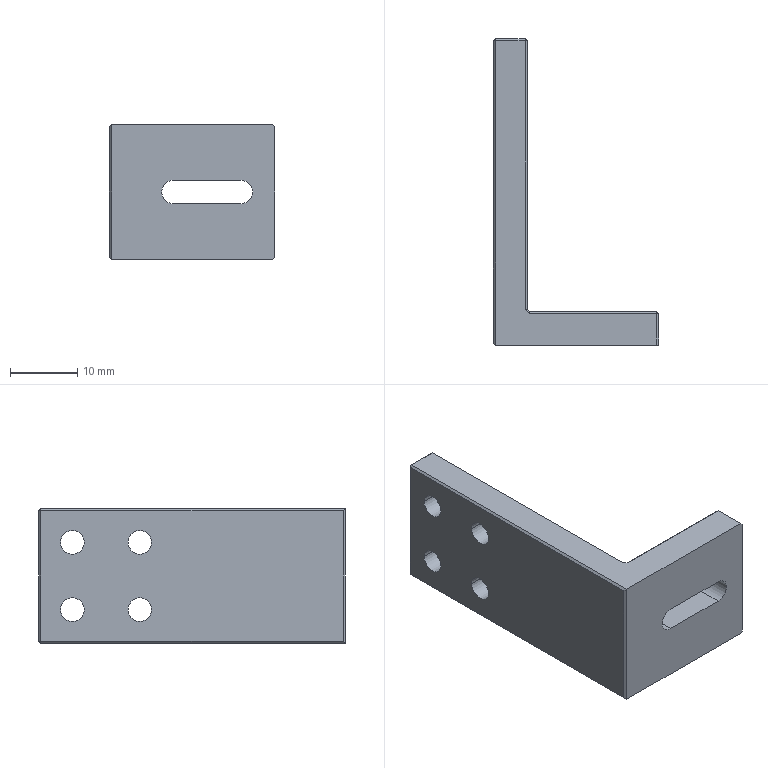Part | SolidWorks | features ICE 2, Chamfer 1, ExtruThin 1 | 1 solid | 43 faces | box 24.5 x 45.5 x 20 mm | volume 6072 mm3 | plane 33 | cylinder 10 | commonest cylinder face diameters 3.5 x10
STEP:
#1=CARTESIAN_POINT('',(0.,42.25,5.));
#2=VERTEX_POINT('',#1);
#3=CARTESIAN_POINT('',(0.,38.75,5.));
#4=VERTEX_POINT('',#3);
#5=CARTESIAN_POINT('',(0.,40.5,5.));
#6=DIRECTION('',(-1.,0.,0.));
#7=DIRECTION('',(0.,1.,0.));
#8=AXIS2_PLACEMENT_3D('',#5,#6,#7);
#9=CIRCLE('',#8,1.75);
#10=EDGE_CURVE('',#2,#4,#9,.T.);
#11=ORIENTED_EDGE('',*,*,#10,.T.);
#12=CARTESIAN_POINT('',(5.,38.75,5.));
#13=VERTEX_POINT('',#12);
#14=CARTESIAN_POINT('',(-0.001,38.75,5.));
#15=DIRECTION('',(1.,0.,0.));
#16=VECTOR('',#15,1000.);
#17=LINE('',#14,#16);
#18=EDGE_CURVE('',#4,#13,#17,.T.);
#19=ORIENTED_EDGE('',*,*,#18,.T.);
#20=CARTESIAN_POINT('',(5.,42.25,5.));
#21=VERTEX_POINT('',#20);
#22=CARTESIAN_POINT('',(5.,40.5,5.));
#23=DIRECTION('',(1.,0.,0.));
#24=DIRECTION('',(0.,-1.,0.));
#25=AXIS2_PLACEMENT_3D('',#22,#23,#24);
#26=CIRCLE('',#25,1.75);
#27=EDGE_CURVE('',#13,#21,#26,.T.);
#28=ORIENTED_EDGE('',*,*,#27,.T.);
#29=CARTESIAN_POINT('',(-0.001,42.25,5.));
#30=DIRECTION('',(1.,0.,0.));
#31=VECTOR('',#30,1000.);
#32=LINE('',#29,#31);
#33=EDGE_CURVE('',#2,#21,#32,.T.);
#34=ORIENTED_EDGE('',*,*,#33,.F.);
#35=EDGE_LOOP('',(#11,#19,#28,#34));
#36=FACE_OUTER_BOUND('',#35,.T.);
#37=CARTESIAN_POINT('',(-0.001,40.5,5.));
#38=DIRECTION('',(1.,0.,0.));
#39=DIRECTION('',(0.,1.,0.));
#40=AXIS2_PLACEMENT_3D('',#37,#38,#39);
#41=CYLINDRICAL_SURFACE('',#40,1.75);
#42=ADVANCED_FACE('',(#36),#41,.F.);
#43=CARTESIAN_POINT('',(0.,32.25,5.));
#44=VERTEX_POINT('',#43);
#45=CARTESIAN_POINT('',(0.,28.75,5.));
#46=VERTEX_POINT('',#45);
#47=CARTESIAN_POINT('',(0.,30.5,5.));
#48=DIRECTION('',(-1.,0.,0.));
#49=DIRECTION('',(0.,1.,0.));
#50=AXIS2_PLACEMENT_3D('',#47,#48,#49);
#51=CIRCLE('',#50,1.75);
#52=EDGE_CURVE('',#44,#46,#51,.T.);
#53=ORIENTED_EDGE('',*,*,#52,.T.);
#54=CARTESIAN_POINT('',(5.,28.75,5.));
#55=VERTEX_POINT('',#54);
#56=CARTESIAN_POINT('',(-0.001,28.75,5.));
#57=DIRECTION('',(1.,0.,0.));
#58=VECTOR('',#57,1000.);
#59=LINE('',#56,#58);
#60=EDGE_CURVE('',#46,#55,#59,.T.);
#61=ORIENTED_EDGE('',*,*,#60,.T.);
#62=CARTESIAN_POINT('',(5.,32.25,5.));
#63=VERTEX_POINT('',#62);
#64=CARTESIAN_POINT('',(5.,30.5,5.));
#65=DIRECTION('',(1.,0.,0.));
#66=DIRECTION('',(0.,-1.,0.));
#67=AXIS2_PLACEMENT_3D('',#64,#65,#66);
#68=CIRCLE('',#67,1.75);
#69=EDGE_CURVE('',#55,#63,#68,.T.);
#70=ORIENTED_EDGE('',*,*,#69,.T.);
#71=CARTESIAN_POINT('',(-0.001,32.25,5.));
#72=DIRECTION('',(1.,0.,0.));
#73=VECTOR('',#72,1000.);
#74=LINE('',#71,#73);
#75=EDGE_CURVE('',#44,#63,#74,.T.);
#76=ORIENTED_EDGE('',*,*,#75,.F.);
#77=EDGE_LOOP('',(#53,#61,#70,#76));
#78=FACE_OUTER_BOUND('',#77,.T.);
#79=CARTESIAN_POINT('',(-0.001,30.5,5.));
#80=DIRECTION('',(1.,0.,0.));
#81=DIRECTION('',(0.,1.,0.));
#82=AXIS2_PLACEMENT_3D('',#79,#80,#81);
#83=CYLINDRICAL_SURFACE('',#82,1.75);
#84=ADVANCED_FACE('',(#78),#83,.F.);
#85=CARTESIAN_POINT('',(0.,32.25,15.));
#86=VERTEX_POINT('',#85);
#87=CARTESIAN_POINT('',(0.,28.75,15.));
#88=VERTEX_POINT('',#87);
#89=CARTESIAN_POINT('',(0.,30.5,15.));
#90=DIRECTION('',(-1.,0.,0.));
#91=DIRECTION('',(0.,1.,0.));
#92=AXIS2_PLACEMENT_3D('',#89,#90,#91);
#93=CIRCLE('',#92,1.75);
#94=EDGE_CURVE('',#86,#88,#93,.T.);
#95=ORIENTED_EDGE('',*,*,#94,.T.);
#96=CARTESIAN_POINT('',(5.,28.75,15.));
#97=VERTEX_POINT('',#96);
#98=CARTESIAN_POINT('',(-0.001,28.75,15.));
#99=DIRECTION('',(1.,0.,0.));
#100=VECTOR('',#99,1000.);
#101=LINE('',#98,#100);
#102=EDGE_CURVE('',#88,#97,#101,.T.);
#103=ORIENTED_EDGE('',*,*,#102,.T.);
#104=CARTESIAN_POINT('',(5.,32.25,15.));
#105=VERTEX_POINT('',#104);
#106=CARTESIAN_POINT('',(5.,30.5,15.));
#107=DIRECTION('',(1.,0.,0.));
#108=DIRECTION('',(0.,1.,0.));
#109=AXIS2_PLACEMENT_3D('',#106,#107,#108);
#110=CIRCLE('',#109,1.75);
#111=EDGE_CURVE('',#97,#105,#110,.T.);
#112=ORIENTED_EDGE('',*,*,#111,.T.);
#113=CARTESIAN_POINT('',(-0.001,32.25,15.));
#114=DIRECTION('',(1.,0.,0.));
#115=VECTOR('',#114,1000.);
#116=LINE('',#113,#115);
#117=EDGE_CURVE('',#86,#105,#116,.T.);
#118=ORIENTED_EDGE('',*,*,#117,.F.);
#119=EDGE_LOOP('',(#95,#103,#112,#118));
#120=FACE_OUTER_BOUND('',#119,.T.);
#121=CARTESIAN_POINT('',(-0.001,30.5,15.));
#122=DIRECTION('',(1.,0.,0.));
#123=DIRECTION('',(0.,1.,0.));
#124=AXIS2_PLACEMENT_3D('',#121,#122,#123);
#125=CYLINDRICAL_SURFACE('',#124,1.75);
#126=ADVANCED_FACE('',(#120),#125,.F.);
#127=CARTESIAN_POINT('',(0.,42.25,15.));
#128=VERTEX_POINT('',#127);
#129=CARTESIAN_POINT('',(0.,38.75,15.));
#130=VERTEX_POINT('',#129);
#131=CARTESIAN_POINT('',(0.,40.5,15.));
#132=DIRECTION('',(-1.,0.,0.));
#133=DIRECTION('',(0.,1.,0.));
#134=AXIS2_PLACEMENT_3D('',#131,#132,#133);
#135=CIRCLE('',#134,1.75);
#136=EDGE_CURVE('',#128,#130,#135,.T.);
#137=ORIENTED_EDGE('',*,*,#136,.T.);
#138=CARTESIAN_POINT('',(5.,38.75,15.));
#139=VERTEX_POINT('',#138);
#140=CARTESIAN_POINT('',(-0.001,38.75,15.));
#141=DIRECTION('',(1.,0.,0.));
#142=VECTOR('',#141,1000.);
#143=LINE('',#140,#142);
#144=EDGE_CURVE('',#130,#139,#143,.T.);
#145=ORIENTED_EDGE('',*,*,#144,.T.);
#146=CARTESIAN_POINT('',(5.,42.25,15.));
#147=VERTEX_POINT('',#146);
#148=CARTESIAN_POINT('',(5.,40.5,15.));
#149=DIRECTION('',(1.,0.,0.));
#150=DIRECTION('',(0.,1.,0.));
#151=AXIS2_PLACEMENT_3D('',#148,#149,#150);
#152=CIRCLE('',#151,1.75);
#153=EDGE_CURVE('',#139,#147,#152,.T.);
#154=ORIENTED_EDGE('',*,*,#153,.T.);
#155=CARTESIAN_POINT('',(-0.001,42.25,15.));
#156=DIRECTION('',(1.,0.,0.));
#157=VECTOR('',#156,1000.);
#158=LINE('',#155,#157);
#159=EDGE_CURVE('',#128,#147,#158,.T.);
#160=ORIENTED_EDGE('',*,*,#159,.F.);
#161=EDGE_LOOP('',(#137,#145,#154,#160));
#162=FACE_OUTER_BOUND('',#161,.T.);
#163=CARTESIAN_POINT('',(-0.001,40.5,15.));
#164=DIRECTION('',(1.,0.,0.));
#165=DIRECTION('',(0.,1.,0.));
#166=AXIS2_PLACEMENT_3D('',#163,#164,#165);
#167=CYLINDRICAL_SURFACE('',#166,1.75);
#168=ADVANCED_FACE('',(#162),#167,.F.);
#169=CARTESIAN_POINT('',(4.7,45.2,20.));
#170=VERTEX_POINT('',#169);
#171=CARTESIAN_POINT('',(0.3,45.2,20.));
#172=VERTEX_POINT('',#171);
#173=CARTESIAN_POINT('',(0.,45.2,20.));
#174=DIRECTION('',(-1.,0.,0.));
#175=VECTOR('',#174,1000.);
#176=LINE('',#173,#175);
#177=EDGE_CURVE('',#170,#172,#176,.T.);
#178=ORIENTED_EDGE('',*,*,#177,.T.);
#179=CARTESIAN_POINT('',(0.3,0.,20.));
#180=VERTEX_POINT('',#179);
#181=CARTESIAN_POINT('',(0.3,0.,20.));
#182=DIRECTION('',(0.,-1.,0.));
#183=VECTOR('',#182,1000.);
#184=LINE('',#181,#183);
#185=EDGE_CURVE('',#172,#180,#184,.T.);
#186=ORIENTED_EDGE('',*,*,#185,.T.);
#187=CARTESIAN_POINT('',(24.2,0.,20.));
#188=VERTEX_POINT('',#187);
#189=CARTESIAN_POINT('',(0.,0.,20.));
#190=DIRECTION('',(1.,0.,0.));
#191=VECTOR('',#190,1000.);
#192=LINE('',#189,#191);
#193=EDGE_CURVE('',#180,#188,#192,.T.);
#194=ORIENTED_EDGE('',*,*,#193,.T.);
#195=CARTESIAN_POINT('',(24.2,4.7,20.));
#196=VERTEX_POINT('',#195);
#197=CARTESIAN_POINT('',(24.2,5.,20.));
#198=DIRECTION('',(0.,1.,0.));
#199=VECTOR('',#198,1000.);
#200=LINE('',#197,#199);
#201=EDGE_CURVE('',#188,#196,#200,.T.);
#202=ORIENTED_EDGE('',*,*,#201,.T.);
#203=CARTESIAN_POINT('',(5.3,4.7,20.));
#204=VERTEX_POINT('',#203);
#205=CARTESIAN_POINT('',(5.,4.7,20.));
#206=DIRECTION('',(-1.,0.,0.));
#207=VECTOR('',#206,1000.);
#208=LINE('',#205,#207);
#209=EDGE_CURVE('',#196,#204,#208,.T.);
#210=ORIENTED_EDGE('',*,*,#209,.T.);
#211=CARTESIAN_POINT('',(4.7,5.3,20.));
#212=VERTEX_POINT('',#211);
#213=CARTESIAN_POINT('',(5.3,4.7,20.));
#214=DIRECTION('',(0.7071,-0.7071,0.));
#215=VECTOR('',#214,1000.);
#216=LINE('',#213,#215);
#217=EDGE_CURVE('',#212,#204,#216,.T.);
#218=ORIENTED_EDGE('',*,*,#217,.F.);
#219=CARTESIAN_POINT('',(4.7,45.5,20.));
#220=DIRECTION('',(0.,1.,0.));
#221=VECTOR('',#220,1000.);
#222=LINE('',#219,#221);
#223=EDGE_CURVE('',#212,#170,#222,.T.);
#224=ORIENTED_EDGE('',*,*,#223,.T.);
#225=EDGE_LOOP('',(#178,#186,#194,#202,#210,#218,#224));
#226=FACE_OUTER_BOUND('',#225,.T.);
#227=CARTESIAN_POINT('',(0.,0.,20.));
#228=DIRECTION('',(0.,0.,-1.));
#229=DIRECTION('',(-1.,0.,0.));
#230=AXIS2_PLACEMENT_3D('',#227,#228,#229);
#231=PLANE('',#230);
#232=ADVANCED_FACE('',(#226),#231,.F.);
#233=CARTESIAN_POINT('',(5.3,4.7,0.));
#234=VERTEX_POINT('',#233);
#235=CARTESIAN_POINT('',(24.2,4.7,0.));
#236=VERTEX_POINT('',#235);
#237=CARTESIAN_POINT('',(0.,4.7,0.));
#238=DIRECTION('',(1.,0.,0.));
#239=VECTOR('',#238,1000.);
#240=LINE('',#237,#239);
#241=EDGE_CURVE('',#234,#236,#240,.T.);
#242=ORIENTED_EDGE('',*,*,#241,.T.);
#243=CARTESIAN_POINT('',(24.2,0.,0.));
#244=VERTEX_POINT('',#243);
#245=CARTESIAN_POINT('',(24.2,0.,0.));
#246=DIRECTION('',(0.,-1.,0.));
#247=VECTOR('',#246,1000.);
#248=LINE('',#245,#247);
#249=EDGE_CURVE('',#236,#244,#248,.T.);
#250=ORIENTED_EDGE('',*,*,#249,.T.);
#251=CARTESIAN_POINT('',(0.3,0.,0.));
#252=VERTEX_POINT('',#251);
#253=CARTESIAN_POINT('',(0.,0.,0.));
#254=DIRECTION('',(1.,0.,0.));
#255=VECTOR('',#254,1000.);
#256=LINE('',#253,#255);
#257=EDGE_CURVE('',#252,#244,#256,.T.);
#258=ORIENTED_EDGE('',*,*,#257,.F.);
#259=CARTESIAN_POINT('',(0.3,45.2,0.));
#260=VERTEX_POINT('',#259);
#261=CARTESIAN_POINT('',(0.3,45.5,0.));
#262=DIRECTION('',(0.,1.,0.));
#263=VECTOR('',#262,1000.);
#264=LINE('',#261,#263);
#265=EDGE_CURVE('',#252,#260,#264,.T.);
#266=ORIENTED_EDGE('',*,*,#265,.T.);
#267=CARTESIAN_POINT('',(4.7,45.2,0.));
#268=VERTEX_POINT('',#267);
#269=CARTESIAN_POINT('',(0.,45.2,0.));
#270=DIRECTION('',(1.,0.,0.));
#271=VECTOR('',#270,1000.);
#272=LINE('',#269,#271);
#273=EDGE_CURVE('',#260,#268,#272,.T.);
#274=ORIENTED_EDGE('',*,*,#273,.T.);
#275=CARTESIAN_POINT('',(4.7,5.3,0.));
#276=VERTEX_POINT('',#275);
#277=CARTESIAN_POINT('',(4.7,0.,0.));
#278=DIRECTION('',(0.,-1.,0.));
#279=VECTOR('',#278,1000.);
#280=LINE('',#277,#279);
#281=EDGE_CURVE('',#268,#276,#280,.T.);
#282=ORIENTED_EDGE('',*,*,#281,.T.);
#283=CARTESIAN_POINT('',(5.,5.,0.));
#284=DIRECTION('',(-0.7071,0.7071,0.));
#285=VECTOR('',#284,1000.);
#286=LINE('',#283,#285);
#287=EDGE_CURVE('',#234,#276,#286,.T.);
#288=ORIENTED_EDGE('',*,*,#287,.F.);
#289=EDGE_LOOP('',(#242,#250,#258,#266,#274,#282,#288));
#290=FACE_OUTER_BOUND('',#289,.T.);
#291=CARTESIAN_POINT('',(0.,0.,0.));
#292=DIRECTION('',(0.,0.,-1.));
#293=DIRECTION('',(-1.,0.,0.));
#294=AXIS2_PLACEMENT_3D('',#291,#292,#293);
#295=PLANE('',#294);
#296=ADVANCED_FACE('',(#290),#295,.T.);
#297=CARTESIAN_POINT('',(9.5,0.,8.25));
#298=VERTEX_POINT('',#297);
#299=CARTESIAN_POINT('',(19.5,0.,8.25));
#300=VERTEX_POINT('',#299);
#301=CARTESIAN_POINT('',(9.5,0.,8.25));
#302=DIRECTION('',(1.,0.,0.));
#303=VECTOR('',#302,1000.);
#304=LINE('',#301,#303);
#305=EDGE_CURVE('',#298,#300,#304,.T.);
#306=ORIENTED_EDGE('',*,*,#305,.F.);
#307=CARTESIAN_POINT('',(9.5,0.,11.75));
#308=VERTEX_POINT('',#307);
#309=CARTESIAN_POINT('',(9.5,0.,10.));
#310=DIRECTION('',(0.,-1.,0.));
#311=DIRECTION('',(0.,0.,1.));
#312=AXIS2_PLACEMENT_3D('',#309,#310,#311);
#313=CIRCLE('',#312,1.75);
#314=EDGE_CURVE('',#308,#298,#313,.T.);
#315=ORIENTED_EDGE('',*,*,#314,.F.);
#316=CARTESIAN_POINT('',(19.5,0.,11.75));
#317=VERTEX_POINT('',#316);
#318=CARTESIAN_POINT('',(9.5,0.,11.75));
#319=DIRECTION('',(-1.,0.,0.));
#320=VECTOR('',#319,1000.);
#321=LINE('',#318,#320);
#322=EDGE_CURVE('',#317,#308,#321,.T.);
#323=ORIENTED_EDGE('',*,*,#322,.F.);
#324=CARTESIAN_POINT('',(19.5,0.,10.));
#325=DIRECTION('',(0.,-1.,0.));
#326=DIRECTION('',(0.,0.,1.));
#327=AXIS2_PLACEMENT_3D('',#324,#325,#326);
#328=CIRCLE('',#327,1.75);
#329=EDGE_CURVE('',#300,#317,#328,.T.);
#330=ORIENTED_EDGE('',*,*,#329,.F.);
#331=EDGE_LOOP('',(#306,#315,#323,#330));
#332=FACE_BOUND('',#331,.T.);
#333=ORIENTED_EDGE('',*,*,#257,.T.);
#334=CARTESIAN_POINT('',(24.5,0.,0.3));
#335=VERTEX_POINT('',#334);
#336=CARTESIAN_POINT('',(24.2,0.,0.));
#337=DIRECTION('',(0.7071,0.,0.7071));
#338=VECTOR('',#337,1000.);
#339=LINE('',#336,#338);
#340=EDGE_CURVE('',#244,#335,#339,.T.);
#341=ORIENTED_EDGE('',*,*,#340,.T.);
#342=CARTESIAN_POINT('',(24.5,0.,19.7));
#343=VERTEX_POINT('',#342);
#344=CARTESIAN_POINT('',(24.5,0.,20.));
#345=DIRECTION('',(0.,0.,-1.));
#346=VECTOR('',#345,1000.);
#347=LINE('',#344,#346);
#348=EDGE_CURVE('',#343,#335,#347,.T.);
#349=ORIENTED_EDGE('',*,*,#348,.F.);
#350=CARTESIAN_POINT('',(24.5,0.,19.7));
#351=DIRECTION('',(-0.7071,0.,0.7071));
#352=VECTOR('',#351,1000.);
#353=LINE('',#350,#352);
#354=EDGE_CURVE('',#343,#188,#353,.T.);
#355=ORIENTED_EDGE('',*,*,#354,.T.);
#356=ORIENTED_EDGE('',*,*,#193,.F.);
#357=CARTESIAN_POINT('',(0.3,0.,20.));
#358=DIRECTION('',(0.,0.,-1.));
#359=VECTOR('',#358,1000.);
#360=LINE('',#357,#359);
#361=EDGE_CURVE('',#180,#252,#360,.T.);
#362=ORIENTED_EDGE('',*,*,#361,.T.);
#363=EDGE_LOOP('',(#333,#341,#349,#355,#356,#362));
#364=FACE_OUTER_BOUND('',#363,.T.);
#365=CARTESIAN_POINT('',(0.,0.,20.));
#366=DIRECTION('',(0.,1.,0.));
#367=DIRECTION('',(0.,0.,1.));
#368=AXIS2_PLACEMENT_3D('',#365,#366,#367);
#369=PLANE('',#368);
#370=ADVANCED_FACE('',(#332,#364),#369,.F.);
#371=ORIENTED_EDGE('',*,*,#348,.T.);
#372=CARTESIAN_POINT('',(24.5,4.7,0.3));
#373=VERTEX_POINT('',#372);
#374=CARTESIAN_POINT('',(24.5,5.,0.3));
#375=DIRECTION('',(0.,1.,0.));
#376=VECTOR('',#375,1000.);
#377=LINE('',#374,#376);
#378=EDGE_CURVE('',#335,#373,#377,.T.);
#379=ORIENTED_EDGE('',*,*,#378,.T.);
#380=CARTESIAN_POINT('',(24.5,4.7,19.7));
#381=VERTEX_POINT('',#380);
#382=CARTESIAN_POINT('',(24.5,4.7,20.));
#383=DIRECTION('',(0.,0.,1.));
#384=VECTOR('',#383,1000.);
#385=LINE('',#382,#384);
#386=EDGE_CURVE('',#373,#381,#385,.T.);
#387=ORIENTED_EDGE('',*,*,#386,.T.);
#388=CARTESIAN_POINT('',(24.5,0.,19.7));
#389=DIRECTION('',(0.,-1.,0.));
#390=VECTOR('',#389,1000.);
#391=LINE('',#388,#390);
#392=EDGE_CURVE('',#381,#343,#391,.T.);
#393=ORIENTED_EDGE('',*,*,#392,.T.);
#394=EDGE_LOOP('',(#371,#379,#387,#393));
#395=FACE_OUTER_BOUND('',#394,.T.);
#396=CARTESIAN_POINT('',(24.5,5.,20.));
#397=DIRECTION('',(1.,0.,0.));
#398=DIRECTION('',(0.,0.,-1.));
#399=AXIS2_PLACEMENT_3D('',#396,#397,#398);
#400=PLANE('',#399);
#401=ADVANCED_FACE('',(#395),#400,.T.);
#402=CARTESIAN_POINT('',(9.5,5.,8.25));
#403=VERTEX_POINT('',#402);
#404=CARTESIAN_POINT('',(9.5,5.,11.75));
#405=VERTEX_POINT('',#404);
#406=CARTESIAN_POINT('',(9.5,5.,10.));
#407=DIRECTION('',(0.,1.,0.));
#408=DIRECTION('',(0.,0.,1.));
#409=AXIS2_PLACEMENT_3D('',#406,#407,#408);
#410=CIRCLE('',#409,1.75);
#411=EDGE_CURVE('',#403,#405,#410,.T.);
#412=ORIENTED_EDGE('',*,*,#411,.F.);
#413=CARTESIAN_POINT('',(19.5,5.,8.25));
#414=VERTEX_POINT('',#413);
#415=CARTESIAN_POINT('',(9.5,5.,8.25));
#416=DIRECTION('',(-1.,0.,0.));
#417=VECTOR('',#416,1000.);
#418=LINE('',#415,#417);
#419=EDGE_CURVE('',#414,#403,#418,.T.);
#420=ORIENTED_EDGE('',*,*,#419,.F.);
#421=CARTESIAN_POINT('',(19.5,5.,11.75));
#422=VERTEX_POINT('',#421);
#423=CARTESIAN_POINT('',(19.5,5.,10.));
#424=DIRECTION('',(0.,1.,0.));
#425=DIRECTION('',(0.,0.,1.));
#426=AXIS2_PLACEMENT_3D('',#423,#424,#425);
#427=CIRCLE('',#426,1.75);
#428=EDGE_CURVE('',#422,#414,#427,.T.);
#429=ORIENTED_EDGE('',*,*,#428,.F.);
#430=CARTESIAN_POINT('',(9.5,5.,11.75));
#431=DIRECTION('',(1.,0.,0.));
#432=VECTOR('',#431,1000.);
#433=LINE('',#430,#432);
#434=EDGE_CURVE('',#405,#422,#433,.T.);
#435=ORIENTED_EDGE('',*,*,#434,.F.);
#436=EDGE_LOOP('',(#412,#420,#429,#435));
#437=FACE_BOUND('',#436,.T.);
#438=CARTESIAN_POINT('',(5.3,5.,19.7));
#439=VERTEX_POINT('',#438);
#440=CARTESIAN_POINT('',(24.2,5.,19.7));
#441=VERTEX_POINT('',#440);
#442=CARTESIAN_POINT('',(24.5,5.,19.7));
#443=DIRECTION('',(1.,0.,0.));
#444=VECTOR('',#443,1000.);
#445=LINE('',#442,#444);
#446=EDGE_CURVE('',#439,#441,#445,.T.);
#447=ORIENTED_EDGE('',*,*,#446,.T.);
#448=CARTESIAN_POINT('',(24.2,5.,0.3));
#449=VERTEX_POINT('',#448);
#450=CARTESIAN_POINT('',(24.2,5.,20.));
#451=DIRECTION('',(0.,0.,-1.));
#452=VECTOR('',#451,1000.);
#453=LINE('',#450,#452);
#454=EDGE_CURVE('',#441,#449,#453,.T.);
#455=ORIENTED_EDGE('',*,*,#454,.T.);
#456=CARTESIAN_POINT('',(5.3,5.,0.3));
#457=VERTEX_POINT('',#456);
#458=CARTESIAN_POINT('',(0.,5.,0.3));
#459=DIRECTION('',(-1.,0.,0.));
#460=VECTOR('',#459,1000.);
#461=LINE('',#458,#460);
#462=EDGE_CURVE('',#449,#457,#461,.T.);
#463=ORIENTED_EDGE('',*,*,#462,.T.);
#464=CARTESIAN_POINT('',(5.3,5.,20.));
#465=DIRECTION('',(0.,0.,1.));
#466=VECTOR('',#465,1000.);
#467=LINE('',#464,#466);
#468=EDGE_CURVE('',#457,#439,#467,.T.);
#469=ORIENTED_EDGE('',*,*,#468,.T.);
#470=EDGE_LOOP('',(#447,#455,#463,#469));
#471=FACE_OUTER_BOUND('',#470,.T.);
#472=CARTESIAN_POINT('',(0.,5.,20.));
#473=DIRECTION('',(0.,1.,0.));
#474=DIRECTION('',(0.,0.,1.));
#475=AXIS2_PLACEMENT_3D('',#472,#473,#474);
#476=PLANE('',#475);
#477=ADVANCED_FACE('',(#437,#471),#476,.T.);
#478=CARTESIAN_POINT('',(5.,40.5,5.));
#479=DIRECTION('',(1.,0.,0.));
#480=DIRECTION('',(0.,-1.,0.));
#481=AXIS2_PLACEMENT_3D('',#478,#479,#480);
#482=CIRCLE('',#481,1.75);
#483=EDGE_CURVE('',#21,#13,#482,.T.);
#484=ORIENTED_EDGE('',*,*,#483,.F.);
#485=ORIENTED_EDGE('',*,*,#27,.F.);
#486=EDGE_LOOP('',(#484,#485));
#487=FACE_BOUND('',#486,.T.);
#488=CARTESIAN_POINT('',(5.,30.5,5.));
#489=DIRECTION('',(1.,0.,0.));
#490=DIRECTION('',(0.,-1.,0.));
#491=AXIS2_PLACEMENT_3D('',#488,#489,#490);
#492=CIRCLE('',#491,1.75);
#493=EDGE_CURVE('',#63,#55,#492,.T.);
#494=ORIENTED_EDGE('',*,*,#493,.F.);
#495=ORIENTED_EDGE('',*,*,#69,.F.);
#496=EDGE_LOOP('',(#494,#495));
#497=FACE_BOUND('',#496,.T.);
#498=CARTESIAN_POINT('',(5.,30.5,15.));
#499=DIRECTION('',(1.,0.,0.));
#500=DIRECTION('',(0.,1.,0.));
#501=AXIS2_PLACEMENT_3D('',#498,#499,#500);
#502=CIRCLE('',#501,1.75);
#503=EDGE_CURVE('',#105,#97,#502,.T.);
#504=ORIENTED_EDGE('',*,*,#503,.F.);
#505=ORIENTED_EDGE('',*,*,#111,.F.);
#506=EDGE_LOOP('',(#504,#505));
#507=FACE_BOUND('',#506,.T.);
#508=CARTESIAN_POINT('',(5.,40.5,15.));
#509=DIRECTION('',(1.,0.,0.));
#510=DIRECTION('',(0.,1.,0.));
#511=AXIS2_PLACEMENT_3D('',#508,#509,#510);
#512=CIRCLE('',#511,1.75);
#513=EDGE_CURVE('',#147,#139,#512,.T.);
#514=ORIENTED_EDGE('',*,*,#513,.F.);
#515=ORIENTED_EDGE('',*,*,#153,.F.);
#516=EDGE_LOOP('',(#514,#515));
#517=FACE_BOUND('',#516,.T.);
#518=CARTESIAN_POINT('',(5.,45.2,19.7));
#519=VERTEX_POINT('',#518);
#520=CARTESIAN_POINT('',(5.,5.3,19.7));
#521=VERTEX_POINT('',#520);
#522=CARTESIAN_POINT('',(5.,5.,19.7));
#523=DIRECTION('',(0.,-1.,0.));
#524=VECTOR('',#523,1000.);
#525=LINE('',#522,#524);
#526=EDGE_CURVE('',#519,#521,#525,.T.);
#527=ORIENTED_EDGE('',*,*,#526,.T.);
#528=CARTESIAN_POINT('',(5.,5.3,0.3));
#529=VERTEX_POINT('',#528);
#530=CARTESIAN_POINT('',(5.,5.3,0.));
#531=DIRECTION('',(0.,0.,-1.));
#532=VECTOR('',#531,1000.);
#533=LINE('',#530,#532);
#534=EDGE_CURVE('',#521,#529,#533,.T.);
#535=ORIENTED_EDGE('',*,*,#534,.T.);
#536=CARTESIAN_POINT('',(5.,45.2,0.3));
#537=VERTEX_POINT('',#536);
#538=CARTESIAN_POINT('',(5.,45.5,0.3));
#539=DIRECTION('',(0.,1.,0.));
#540=VECTOR('',#539,1000.);
#541=LINE('',#538,#540);
#542=EDGE_CURVE('',#529,#537,#541,.T.);
#543=ORIENTED_EDGE('',*,*,#542,.T.);
#544=CARTESIAN_POINT('',(5.,45.2,20.));
#545=DIRECTION('',(0.,0.,1.));
#546=VECTOR('',#545,1000.);
#547=LINE('',#544,#546);
#548=EDGE_CURVE('',#537,#519,#547,.T.);
#549=ORIENTED_EDGE('',*,*,#548,.T.);
#550=EDGE_LOOP('',(#527,#535,#543,#549));
#551=FACE_OUTER_BOUND('',#550,.T.);
#552=CARTESIAN_POINT('',(5.,45.5,20.));
#553=DIRECTION('',(1.,0.,0.));
#554=DIRECTION('',(0.,1.,0.));
#555=AXIS2_PLACEMENT_3D('',#552,#553,#554);
#556=PLANE('',#555);
#557=ADVANCED_FACE('',(#487,#497,#507,#517,#551),#556,.T.);
#558=CARTESIAN_POINT('',(0.3,45.5,19.7));
#559=VERTEX_POINT('',#558);
#560=CARTESIAN_POINT('',(4.7,45.5,19.7));
#561=VERTEX_POINT('',#560);
#562=CARTESIAN_POINT('',(5.,45.5,19.7));
#563=DIRECTION('',(1.,0.,0.));
#564=VECTOR('',#563,1000.);
#565=LINE('',#562,#564);
#566=EDGE_CURVE('',#559,#561,#565,.T.);
#567=ORIENTED_EDGE('',*,*,#566,.T.);
#568=CARTESIAN_POINT('',(4.7,45.5,0.3));
#569=VERTEX_POINT('',#568);
#570=CARTESIAN_POINT('',(4.7,45.5,20.));
#571=DIRECTION('',(0.,0.,-1.));
#572=VECTOR('',#571,1000.);
#573=LINE('',#570,#572);
#574=EDGE_CURVE('',#561,#569,#573,.T.);
#575=ORIENTED_EDGE('',*,*,#574,.T.);
#576=CARTESIAN_POINT('',(0.3,45.5,0.3));
#577=VERTEX_POINT('',#576);
#578=CARTESIAN_POINT('',(0.,45.5,0.3));
#579=DIRECTION('',(-1.,0.,0.));
#580=VECTOR('',#579,1000.);
#581=LINE('',#578,#580);
#582=EDGE_CURVE('',#569,#577,#581,.T.);
#583=ORIENTED_EDGE('',*,*,#582,.T.);
#584=CARTESIAN_POINT('',(0.3,45.5,20.));
#585=DIRECTION('',(0.,0.,1.));
#586=VECTOR('',#585,1000.);
#587=LINE('',#584,#586);
#588=EDGE_CURVE('',#577,#559,#587,.T.);
#589=ORIENTED_EDGE('',*,*,#588,.T.);
#590=EDGE_LOOP('',(#567,#575,#583,#589));
#591=FACE_OUTER_BOUND('',#590,.T.);
#592=CARTESIAN_POINT('',(0.,45.5,20.));
#593=DIRECTION('',(0.,1.,0.));
#594=DIRECTION('',(0.,0.,1.));
#595=AXIS2_PLACEMENT_3D('',#592,#593,#594);
#596=PLANE('',#595);
#597=ADVANCED_FACE('',(#591),#596,.T.);
#598=ORIENTED_EDGE('',*,*,#10,.F.);
#599=CARTESIAN_POINT('',(0.,40.5,5.));
#600=DIRECTION('',(-1.,0.,0.));
#601=DIRECTION('',(0.,1.,0.));
#602=AXIS2_PLACEMENT_3D('',#599,#600,#601);
#603=CIRCLE('',#602,1.75);
#604=EDGE_CURVE('',#4,#2,#603,.T.);
#605=ORIENTED_EDGE('',*,*,#604,.F.);
#606=EDGE_LOOP('',(#598,#605));
#607=FACE_BOUND('',#606,.T.);
#608=ORIENTED_EDGE('',*,*,#52,.F.);
#609=CARTESIAN_POINT('',(0.,30.5,5.));
#610=DIRECTION('',(-1.,0.,0.));
#611=DIRECTION('',(0.,1.,0.));
#612=AXIS2_PLACEMENT_3D('',#609,#610,#611);
#613=CIRCLE('',#612,1.75);
#614=EDGE_CURVE('',#46,#44,#613,.T.);
#615=ORIENTED_EDGE('',*,*,#614,.F.);
#616=EDGE_LOOP('',(#608,#615));
#617=FACE_BOUND('',#616,.T.);
#618=ORIENTED_EDGE('',*,*,#94,.F.);
#619=CARTESIAN_POINT('',(0.,30.5,15.));
#620=DIRECTION('',(-1.,0.,0.));
#621=DIRECTION('',(0.,1.,0.));
#622=AXIS2_PLACEMENT_3D('',#619,#620,#621);
#623=CIRCLE('',#622,1.75);
#624=EDGE_CURVE('',#88,#86,#623,.T.);
#625=ORIENTED_EDGE('',*,*,#624,.F.);
#626=EDGE_LOOP('',(#618,#625));
#627=FACE_BOUND('',#626,.T.);
#628=ORIENTED_EDGE('',*,*,#136,.F.);
#629=CARTESIAN_POINT('',(0.,40.5,15.));
#630=DIRECTION('',(-1.,0.,0.));
#631=DIRECTION('',(0.,1.,0.));
#632=AXIS2_PLACEMENT_3D('',#629,#630,#631);
#633=CIRCLE('',#632,1.75);
#634=EDGE_CURVE('',#130,#128,#633,.T.);
#635=ORIENTED_EDGE('',*,*,#634,.F.);
#636=EDGE_LOOP('',(#628,#635));
#637=FACE_BOUND('',#636,.T.);
#638=CARTESIAN_POINT('',(0.,0.3,0.3));
#639=VERTEX_POINT('',#638);
#640=CARTESIAN_POINT('',(0.,0.3,19.7));
#641=VERTEX_POINT('',#640);
#642=CARTESIAN_POINT('',(0.,0.3,20.));
#643=DIRECTION('',(0.,0.,1.));
#644=VECTOR('',#643,1000.);
#645=LINE('',#642,#644);
#646=EDGE_CURVE('',#639,#641,#645,.T.);
#647=ORIENTED_EDGE('',*,*,#646,.T.);
#648=CARTESIAN_POINT('',(0.,45.2,19.7));
#649=VERTEX_POINT('',#648);
#650=CARTESIAN_POINT('',(0.,45.5,19.7));
#651=DIRECTION('',(0.,1.,0.));
#652=VECTOR('',#651,1000.);
#653=LINE('',#650,#652);
#654=EDGE_CURVE('',#641,#649,#653,.T.);
#655=ORIENTED_EDGE('',*,*,#654,.T.);
#656=CARTESIAN_POINT('',(0.,45.2,0.3));
#657=VERTEX_POINT('',#656);
#658=CARTESIAN_POINT('',(0.,45.2,0.));
#659=DIRECTION('',(0.,0.,-1.));
#660=VECTOR('',#659,1000.);
#661=LINE('',#658,#660);
#662=EDGE_CURVE('',#649,#657,#661,.T.);
#663=ORIENTED_EDGE('',*,*,#662,.T.);
#664=CARTESIAN_POINT('',(0.,0.,0.3));
#665=DIRECTION('',(0.,-1.,0.));
#666=VECTOR('',#665,1000.);
#667=LINE('',#664,#666);
#668=EDGE_CURVE('',#657,#639,#667,.T.);
#669=ORIENTED_EDGE('',*,*,#668,.T.);
#670=EDGE_LOOP('',(#647,#655,#663,#669));
#671=FACE_OUTER_BOUND('',#670,.T.);
#672=CARTESIAN_POINT('',(0.,45.5,20.));
#673=DIRECTION('',(1.,0.,0.));
#674=DIRECTION('',(0.,1.,0.));
#675=AXIS2_PLACEMENT_3D('',#672,#673,#674);
#676=PLANE('',#675);
#677=ADVANCED_FACE('',(#607,#617,#627,#637,#671),#676,.F.);
#678=CARTESIAN_POINT('',(-15.067,15.367,15.367));
#679=DIRECTION('',(-0.5774,0.5774,0.5774));
#680=VECTOR('',#679,1000.);
#681=LINE('',#678,#680);
#682=EDGE_CURVE('',#252,#639,#681,.T.);
#683=ORIENTED_EDGE('',*,*,#682,.F.);
#684=ORIENTED_EDGE('',*,*,#361,.F.);
#685=CARTESIAN_POINT('',(0.3,0.,20.));
#686=DIRECTION('',(0.5774,-0.5774,0.5774));
#687=VECTOR('',#686,1000.);
#688=LINE('',#685,#687);
#689=EDGE_CURVE('',#641,#180,#688,.T.);
#690=ORIENTED_EDGE('',*,*,#689,.F.);
#691=ORIENTED_EDGE('',*,*,#646,.F.);
#692=EDGE_LOOP('',(#683,#684,#690,#691));
#693=FACE_OUTER_BOUND('',#692,.T.);
#694=CARTESIAN_POINT('',(0.3,0.,20.));
#695=DIRECTION('',(0.7071,0.7071,0.));
#696=DIRECTION('',(0.,0.,-1.));
#697=AXIS2_PLACEMENT_3D('',#694,#695,#696);
#698=PLANE('',#697);
#699=ADVANCED_FACE('',(#693),#698,.F.);
#700=ORIENTED_EDGE('',*,*,#689,.T.);
#701=ORIENTED_EDGE('',*,*,#185,.F.);
#702=CARTESIAN_POINT('',(0.,45.2,19.7));
#703=DIRECTION('',(0.7071,0.,0.7071));
#704=VECTOR('',#703,1000.);
#705=LINE('',#702,#704);
#706=EDGE_CURVE('',#649,#172,#705,.T.);
#707=ORIENTED_EDGE('',*,*,#706,.F.);
#708=ORIENTED_EDGE('',*,*,#654,.F.);
#709=EDGE_LOOP('',(#700,#701,#707,#708));
#710=FACE_OUTER_BOUND('',#709,.T.);
#711=CARTESIAN_POINT('',(0.3,0.,20.));
#712=DIRECTION('',(0.7071,0.,-0.7071));
#713=DIRECTION('',(0.,-1.,0.));
#714=AXIS2_PLACEMENT_3D('',#711,#712,#713);
#715=PLANE('',#714);
#716=ADVANCED_FACE('',(#710),#715,.F.);
#717=CARTESIAN_POINT('',(0.15,45.35,0.3));
#718=DIRECTION('',(0.7071,0.7071,0.));
#719=VECTOR('',#718,1000.);
#720=LINE('',#717,#719);
#721=EDGE_CURVE('',#657,#577,#720,.T.);
#722=ORIENTED_EDGE('',*,*,#721,.F.);
#723=ORIENTED_EDGE('',*,*,#662,.F.);
#724=CARTESIAN_POINT('',(0.,45.2,19.7));
#725=DIRECTION('',(-0.7071,-0.7071,0.));
#726=VECTOR('',#725,1000.);
#727=LINE('',#724,#726);
#728=EDGE_CURVE('',#559,#649,#727,.T.);
#729=ORIENTED_EDGE('',*,*,#728,.F.);
#730=ORIENTED_EDGE('',*,*,#588,.F.);
#731=EDGE_LOOP('',(#722,#723,#729,#730));
#732=FACE_OUTER_BOUND('',#731,.T.);
#733=CARTESIAN_POINT('',(0.,45.2,20.));
#734=DIRECTION('',(-0.7071,0.7071,0.));
#735=DIRECTION('',(0.,0.,1.));
#736=AXIS2_PLACEMENT_3D('',#733,#734,#735);
#737=PLANE('',#736);
#738=ADVANCED_FACE('',(#732),#737,.T.);
#739=ORIENTED_EDGE('',*,*,#682,.T.);
#740=ORIENTED_EDGE('',*,*,#668,.F.);
#741=CARTESIAN_POINT('',(0.3,45.2,0.));
#742=DIRECTION('',(-0.7071,0.,0.7071));
#743=VECTOR('',#742,1000.);
#744=LINE('',#741,#743);
#745=EDGE_CURVE('',#260,#657,#744,.T.);
#746=ORIENTED_EDGE('',*,*,#745,.F.);
#747=ORIENTED_EDGE('',*,*,#265,.F.);
#748=EDGE_LOOP('',(#739,#740,#746,#747));
#749=FACE_OUTER_BOUND('',#748,.T.);
#750=CARTESIAN_POINT('',(0.,45.5,0.3));
#751=DIRECTION('',(-0.7071,0.,-0.7071));
#752=DIRECTION('',(0.,1.,0.));
#753=AXIS2_PLACEMENT_3D('',#750,#751,#752);
#754=PLANE('',#753);
#755=ADVANCED_FACE('',(#749),#754,.T.);
#756=ORIENTED_EDGE('',*,*,#728,.T.);
#757=ORIENTED_EDGE('',*,*,#706,.T.);
#758=CARTESIAN_POINT('',(0.3,45.35,19.85));
#759=DIRECTION('',(0.,-0.7071,0.7071));
#760=VECTOR('',#759,1000.);
#761=LINE('',#758,#760);
#762=EDGE_CURVE('',#559,#172,#761,.T.);
#763=ORIENTED_EDGE('',*,*,#762,.F.);
#764=EDGE_LOOP('',(#756,#757,#763));
#765=FACE_OUTER_BOUND('',#764,.T.);
#766=CARTESIAN_POINT('',(0.,45.2,19.7));
#767=DIRECTION('',(-0.5774,0.5774,0.5774));
#768=DIRECTION('',(0.7071,0.,0.7071));
#769=AXIS2_PLACEMENT_3D('',#766,#767,#768);
#770=PLANE('',#769);
#771=ADVANCED_FACE('',(#765),#770,.T.);
#772=ORIENTED_EDGE('',*,*,#745,.T.);
#773=ORIENTED_EDGE('',*,*,#721,.T.);
#774=CARTESIAN_POINT('',(0.3,45.2,0.));
#775=DIRECTION('',(0.,0.7071,0.7071));
#776=VECTOR('',#775,1000.);
#777=LINE('',#774,#776);
#778=EDGE_CURVE('',#260,#577,#777,.T.);
#779=ORIENTED_EDGE('',*,*,#778,.F.);
#780=EDGE_LOOP('',(#772,#773,#779));
#781=FACE_OUTER_BOUND('',#780,.T.);
#782=CARTESIAN_POINT('',(0.3,45.2,0.));
#783=DIRECTION('',(-0.5774,0.5774,-0.5774));
#784=DIRECTION('',(-0.7071,0.,0.7071));
#785=AXIS2_PLACEMENT_3D('',#782,#783,#784);
#786=PLANE('',#785);
#787=ADVANCED_FACE('',(#781),#786,.T.);
#788=ORIENTED_EDGE('',*,*,#762,.T.);
#789=ORIENTED_EDGE('',*,*,#177,.F.);
#790=CARTESIAN_POINT('',(4.7,45.35,19.85));
#791=DIRECTION('',(0.,-0.7071,0.7071));
#792=VECTOR('',#791,1000.);
#793=LINE('',#790,#792);
#794=EDGE_CURVE('',#561,#170,#793,.T.);
#795=ORIENTED_EDGE('',*,*,#794,.F.);
#796=ORIENTED_EDGE('',*,*,#566,.F.);
#797=EDGE_LOOP('',(#788,#789,#795,#796));
#798=FACE_OUTER_BOUND('',#797,.T.);
#799=CARTESIAN_POINT('',(0.,45.5,19.7));
#800=DIRECTION('',(0.,0.7071,0.7071));
#801=DIRECTION('',(-1.,0.,0.));
#802=AXIS2_PLACEMENT_3D('',#799,#800,#801);
#803=PLANE('',#802);
#804=ADVANCED_FACE('',(#798),#803,.T.);
#805=CARTESIAN_POINT('',(5.,45.2,0.3));
#806=DIRECTION('',(0.7071,-0.7071,0.));
#807=VECTOR('',#806,1000.);
#808=LINE('',#805,#807);
#809=EDGE_CURVE('',#569,#537,#808,.T.);
#810=ORIENTED_EDGE('',*,*,#809,.F.);
#811=ORIENTED_EDGE('',*,*,#574,.F.);
#812=CARTESIAN_POINT('',(5.,45.2,19.7));
#813=DIRECTION('',(-0.7071,0.7071,0.));
#814=VECTOR('',#813,1000.);
#815=LINE('',#812,#814);
#816=EDGE_CURVE('',#519,#561,#815,.T.);
#817=ORIENTED_EDGE('',*,*,#816,.F.);
#818=ORIENTED_EDGE('',*,*,#548,.F.);
#819=EDGE_LOOP('',(#810,#811,#817,#818));
#820=FACE_OUTER_BOUND('',#819,.T.);
#821=CARTESIAN_POINT('',(4.7,45.5,20.));
#822=DIRECTION('',(-0.7071,-0.7071,0.));
#823=DIRECTION('',(0.,0.,-1.));
#824=AXIS2_PLACEMENT_3D('',#821,#822,#823);
#825=PLANE('',#824);
#826=ADVANCED_FACE('',(#820),#825,.F.);
#827=ORIENTED_EDGE('',*,*,#778,.T.);
#828=ORIENTED_EDGE('',*,*,#582,.F.);
#829=CARTESIAN_POINT('',(4.7,45.35,0.15));
#830=DIRECTION('',(0.,0.7071,0.7071));
#831=VECTOR('',#830,1000.);
#832=LINE('',#829,#831);
#833=EDGE_CURVE('',#268,#569,#832,.T.);
#834=ORIENTED_EDGE('',*,*,#833,.F.);
#835=ORIENTED_EDGE('',*,*,#273,.F.);
#836=EDGE_LOOP('',(#827,#828,#834,#835));
#837=FACE_OUTER_BOUND('',#836,.T.);
#838=CARTESIAN_POINT('',(0.,45.2,0.));
#839=DIRECTION('',(0.,-0.7071,0.7071));
#840=DIRECTION('',(1.,0.,0.));
#841=AXIS2_PLACEMENT_3D('',#838,#839,#840);
#842=PLANE('',#841);
#843=ADVANCED_FACE('',(#837),#842,.F.);
#844=ORIENTED_EDGE('',*,*,#816,.T.);
#845=ORIENTED_EDGE('',*,*,#794,.T.);
#846=CARTESIAN_POINT('',(5.,45.2,19.7));
#847=DIRECTION('',(-0.7071,0.,0.7071));
#848=VECTOR('',#847,1000.);
#849=LINE('',#846,#848);
#850=EDGE_CURVE('',#519,#170,#849,.T.);
#851=ORIENTED_EDGE('',*,*,#850,.F.);
#852=EDGE_LOOP('',(#844,#845,#851));
#853=FACE_OUTER_BOUND('',#852,.T.);
#854=CARTESIAN_POINT('',(5.,45.2,19.7));
#855=DIRECTION('',(0.5774,0.5774,0.5774));
#856=DIRECTION('',(0.7071,0.,-0.7071));
#857=AXIS2_PLACEMENT_3D('',#854,#855,#856);
#858=PLANE('',#857);
#859=ADVANCED_FACE('',(#853),#858,.T.);
#860=ORIENTED_EDGE('',*,*,#833,.T.);
#861=ORIENTED_EDGE('',*,*,#809,.T.);
#862=CARTESIAN_POINT('',(5.,45.2,0.3));
#863=DIRECTION('',(0.7071,0.,0.7071));
#864=VECTOR('',#863,1000.);
#865=LINE('',#862,#864);
#866=EDGE_CURVE('',#268,#537,#865,.T.);
#867=ORIENTED_EDGE('',*,*,#866,.F.);
#868=EDGE_LOOP('',(#860,#861,#867));
#869=FACE_OUTER_BOUND('',#868,.T.);
#870=CARTESIAN_POINT('',(5.,45.2,0.3));
#871=DIRECTION('',(0.5774,0.5774,-0.5774));
#872=DIRECTION('',(-0.7071,0.,-0.7071));
#873=AXIS2_PLACEMENT_3D('',#870,#871,#872);
#874=PLANE('',#873);
#875=ADVANCED_FACE('',(#869),#874,.T.);
#876=ORIENTED_EDGE('',*,*,#850,.T.);
#877=ORIENTED_EDGE('',*,*,#223,.F.);
#878=CARTESIAN_POINT('',(5.,5.3,19.7));
#879=DIRECTION('',(-0.7071,0.,0.7071));
#880=VECTOR('',#879,1000.);
#881=LINE('',#878,#880);
#882=EDGE_CURVE('',#521,#212,#881,.T.);
#883=ORIENTED_EDGE('',*,*,#882,.F.);
#884=ORIENTED_EDGE('',*,*,#526,.F.);
#885=EDGE_LOOP('',(#876,#877,#883,#884));
#886=FACE_OUTER_BOUND('',#885,.T.);
#887=CARTESIAN_POINT('',(5.,45.5,19.7));
#888=DIRECTION('',(0.7071,0.,0.7071));
#889=DIRECTION('',(0.,1.,0.));
#890=AXIS2_PLACEMENT_3D('',#887,#888,#889);
#891=PLANE('',#890);
#892=ADVANCED_FACE('',(#886),#891,.T.);
#893=CARTESIAN_POINT('',(5.,5.3,0.3));
#894=DIRECTION('',(0.7071,-0.7071,0.));
#895=VECTOR('',#894,1000.);
#896=LINE('',#893,#895);
#897=EDGE_CURVE('',#529,#457,#896,.T.);
#898=ORIENTED_EDGE('',*,*,#897,.F.);
#899=ORIENTED_EDGE('',*,*,#534,.F.);
#900=CARTESIAN_POINT('',(5.3,5.,19.7));
#901=DIRECTION('',(-0.7071,0.7071,0.));
#902=VECTOR('',#901,1000.);
#903=LINE('',#900,#902);
#904=EDGE_CURVE('',#439,#521,#903,.T.);
#905=ORIENTED_EDGE('',*,*,#904,.F.);
#906=ORIENTED_EDGE('',*,*,#468,.F.);
#907=EDGE_LOOP('',(#898,#899,#905,#906));
#908=FACE_OUTER_BOUND('',#907,.T.);
#909=CARTESIAN_POINT('',(5.,5.3,20.));
#910=DIRECTION('',(0.7071,0.7071,0.));
#911=DIRECTION('',(0.,0.,1.));
#912=AXIS2_PLACEMENT_3D('',#909,#910,#911);
#913=PLANE('',#912);
#914=ADVANCED_FACE('',(#908),#913,.T.);
#915=ORIENTED_EDGE('',*,*,#866,.T.);
#916=ORIENTED_EDGE('',*,*,#542,.F.);
#917=CARTESIAN_POINT('',(4.7,5.3,0.));
#918=DIRECTION('',(0.7071,0.,0.7071));
#919=VECTOR('',#918,1000.);
#920=LINE('',#917,#919);
#921=EDGE_CURVE('',#276,#529,#920,.T.);
#922=ORIENTED_EDGE('',*,*,#921,.F.);
#923=ORIENTED_EDGE('',*,*,#281,.F.);
#924=EDGE_LOOP('',(#915,#916,#922,#923));
#925=FACE_OUTER_BOUND('',#924,.T.);
#926=CARTESIAN_POINT('',(4.7,0.,0.));
#927=DIRECTION('',(-0.7071,0.,0.7071));
#928=DIRECTION('',(0.,-1.,0.));
#929=AXIS2_PLACEMENT_3D('',#926,#927,#928);
#930=PLANE('',#929);
#931=ADVANCED_FACE('',(#925),#930,.F.);
#932=ORIENTED_EDGE('',*,*,#882,.T.);
#933=ORIENTED_EDGE('',*,*,#217,.T.);
#934=CARTESIAN_POINT('',(5.3,4.7,20.));
#935=DIRECTION('',(0.,-0.7071,0.7071));
#936=VECTOR('',#935,1000.);
#937=LINE('',#934,#936);
#938=EDGE_CURVE('',#439,#204,#937,.T.);
#939=ORIENTED_EDGE('',*,*,#938,.F.);
#940=ORIENTED_EDGE('',*,*,#904,.T.);
#941=EDGE_LOOP('',(#932,#933,#939,#940));
#942=FACE_OUTER_BOUND('',#941,.T.);
#943=CARTESIAN_POINT('',(5.3,5.,19.7));
#944=DIRECTION('',(0.5774,0.5774,0.5774));
#945=DIRECTION('',(0.,-0.7071,0.7071));
#946=AXIS2_PLACEMENT_3D('',#943,#944,#945);
#947=PLANE('',#946);
#948=ADVANCED_FACE('',(#942),#947,.T.);
#949=ORIENTED_EDGE('',*,*,#921,.T.);
#950=ORIENTED_EDGE('',*,*,#897,.T.);
#951=CARTESIAN_POINT('',(5.3,5.,0.3));
#952=DIRECTION('',(0.,0.7071,0.7071));
#953=VECTOR('',#952,1000.);
#954=LINE('',#951,#953);
#955=EDGE_CURVE('',#234,#457,#954,.T.);
#956=ORIENTED_EDGE('',*,*,#955,.F.);
#957=ORIENTED_EDGE('',*,*,#287,.T.);
#958=EDGE_LOOP('',(#949,#950,#956,#957));
#959=FACE_OUTER_BOUND('',#958,.T.);
#960=CARTESIAN_POINT('',(5.,5.3,0.3));
#961=DIRECTION('',(0.5774,0.5774,-0.5774));
#962=DIRECTION('',(-0.7071,0.7071,0.));
#963=AXIS2_PLACEMENT_3D('',#960,#961,#962);
#964=PLANE('',#963);
#965=ADVANCED_FACE('',(#959),#964,.T.);
#966=ORIENTED_EDGE('',*,*,#354,.F.);
#967=ORIENTED_EDGE('',*,*,#392,.F.);
#968=CARTESIAN_POINT('',(24.5,4.7,19.7));
#969=DIRECTION('',(0.7071,0.,-0.7071));
#970=VECTOR('',#969,1000.);
#971=LINE('',#968,#970);
#972=EDGE_CURVE('',#196,#381,#971,.T.);
#973=ORIENTED_EDGE('',*,*,#972,.F.);
#974=ORIENTED_EDGE('',*,*,#201,.F.);
#975=EDGE_LOOP('',(#966,#967,#973,#974));
#976=FACE_OUTER_BOUND('',#975,.T.);
#977=CARTESIAN_POINT('',(24.5,5.,19.7));
#978=DIRECTION('',(0.7071,0.,0.7071));
#979=DIRECTION('',(0.,1.,0.));
#980=AXIS2_PLACEMENT_3D('',#977,#978,#979);
#981=PLANE('',#980);
#982=ADVANCED_FACE('',(#976),#981,.T.);
#983=ORIENTED_EDGE('',*,*,#938,.T.);
#984=ORIENTED_EDGE('',*,*,#209,.F.);
#985=CARTESIAN_POINT('',(24.2,4.85,19.85));
#986=DIRECTION('',(0.,-0.7071,0.7071));
#987=VECTOR('',#986,1000.);
#988=LINE('',#985,#987);
#989=EDGE_CURVE('',#441,#196,#988,.T.);
#990=ORIENTED_EDGE('',*,*,#989,.F.);
#991=ORIENTED_EDGE('',*,*,#446,.F.);
#992=EDGE_LOOP('',(#983,#984,#990,#991));
#993=FACE_OUTER_BOUND('',#992,.T.);
#994=CARTESIAN_POINT('',(0.,5.,19.7));
#995=DIRECTION('',(0.,0.7071,0.7071));
#996=DIRECTION('',(-1.,0.,0.));
#997=AXIS2_PLACEMENT_3D('',#994,#995,#996);
#998=PLANE('',#997);
#999=ADVANCED_FACE('',(#993),#998,.T.);
#1000=ORIENTED_EDGE('',*,*,#955,.T.);
#1001=ORIENTED_EDGE('',*,*,#462,.F.);
#1002=CARTESIAN_POINT('',(24.2,5.,0.3));
#1003=DIRECTION('',(0.,0.7071,0.7071));
#1004=VECTOR('',#1003,1000.);
#1005=LINE('',#1002,#1004);
#1006=EDGE_CURVE('',#236,#449,#1005,.T.);
#1007=ORIENTED_EDGE('',*,*,#1006,.F.);
#1008=ORIENTED_EDGE('',*,*,#241,.F.);
#1009=EDGE_LOOP('',(#1000,#1001,#1007,#1008));
#1010=FACE_OUTER_BOUND('',#1009,.T.);
#1011=CARTESIAN_POINT('',(0.,4.7,0.));
#1012=DIRECTION('',(0.,-0.7071,0.7071));
#1013=DIRECTION('',(1.,0.,0.));
#1014=AXIS2_PLACEMENT_3D('',#1011,#1012,#1013);
#1015=PLANE('',#1014);
#1016=ADVANCED_FACE('',(#1010),#1015,.F.);
#1017=ORIENTED_EDGE('',*,*,#340,.F.);
#1018=ORIENTED_EDGE('',*,*,#249,.F.);
#1019=CARTESIAN_POINT('',(24.35,4.7,0.15));
#1020=DIRECTION('',(-0.7071,0.,-0.7071));
#1021=VECTOR('',#1020,1000.);
#1022=LINE('',#1019,#1021);
#1023=EDGE_CURVE('',#373,#236,#1022,.T.);
#1024=ORIENTED_EDGE('',*,*,#1023,.F.);
#1025=ORIENTED_EDGE('',*,*,#378,.F.);
#1026=EDGE_LOOP('',(#1017,#1018,#1024,#1025));
#1027=FACE_OUTER_BOUND('',#1026,.T.);
#1028=CARTESIAN_POINT('',(24.2,0.,0.));
#1029=DIRECTION('',(-0.7071,0.,0.7071));
#1030=DIRECTION('',(0.,-1.,0.));
#1031=AXIS2_PLACEMENT_3D('',#1028,#1029,#1030);
#1032=PLANE('',#1031);
#1033=ADVANCED_FACE('',(#1027),#1032,.F.);
#1034=ORIENTED_EDGE('',*,*,#989,.T.);
#1035=ORIENTED_EDGE('',*,*,#972,.T.);
#1036=CARTESIAN_POINT('',(24.5,4.7,19.7));
#1037=DIRECTION('',(0.7071,-0.7071,0.));
#1038=VECTOR('',#1037,1000.);
#1039=LINE('',#1036,#1038);
#1040=EDGE_CURVE('',#441,#381,#1039,.T.);
#1041=ORIENTED_EDGE('',*,*,#1040,.F.);
#1042=EDGE_LOOP('',(#1034,#1035,#1041));
#1043=FACE_OUTER_BOUND('',#1042,.T.);
#1044=CARTESIAN_POINT('',(24.5,4.7,19.7));
#1045=DIRECTION('',(0.5774,0.5774,0.5774));
#1046=DIRECTION('',(0.7071,0.,-0.7071));
#1047=AXIS2_PLACEMENT_3D('',#1044,#1045,#1046);
#1048=PLANE('',#1047);
#1049=ADVANCED_FACE('',(#1043),#1048,.T.);
#1050=ORIENTED_EDGE('',*,*,#1023,.T.);
#1051=ORIENTED_EDGE('',*,*,#1006,.T.);
#1052=CARTESIAN_POINT('',(24.2,5.,0.3));
#1053=DIRECTION('',(-0.7071,0.7071,0.));
#1054=VECTOR('',#1053,1000.);
#1055=LINE('',#1052,#1054);
#1056=EDGE_CURVE('',#373,#449,#1055,.T.);
#1057=ORIENTED_EDGE('',*,*,#1056,.F.);
#1058=EDGE_LOOP('',(#1050,#1051,#1057));
#1059=FACE_OUTER_BOUND('',#1058,.T.);
#1060=CARTESIAN_POINT('',(24.2,5.,0.3));
#1061=DIRECTION('',(0.5774,0.5774,-0.5774));
#1062=DIRECTION('',(-0.7071,0.,-0.7071));
#1063=AXIS2_PLACEMENT_3D('',#1060,#1061,#1062);
#1064=PLANE('',#1063);
#1065=ADVANCED_FACE('',(#1059),#1064,.T.);
#1066=ORIENTED_EDGE('',*,*,#1040,.T.);
#1067=ORIENTED_EDGE('',*,*,#386,.F.);
#1068=ORIENTED_EDGE('',*,*,#1056,.T.);
#1069=ORIENTED_EDGE('',*,*,#454,.F.);
#1070=EDGE_LOOP('',(#1066,#1067,#1068,#1069));
#1071=FACE_OUTER_BOUND('',#1070,.T.);
#1072=CARTESIAN_POINT('',(24.2,5.,20.));
#1073=DIRECTION('',(-0.7071,-0.7071,0.));
#1074=DIRECTION('',(0.,0.,-1.));
#1075=AXIS2_PLACEMENT_3D('',#1072,#1073,#1074);
#1076=PLANE('',#1075);
#1077=ADVANCED_FACE('',(#1071),#1076,.F.);
#1078=ORIENTED_EDGE('',*,*,#314,.T.);
#1079=CARTESIAN_POINT('',(9.5,-0.001,8.25));
#1080=DIRECTION('',(0.,1.,0.));
#1081=VECTOR('',#1080,1000.);
#1082=LINE('',#1079,#1081);
#1083=EDGE_CURVE('',#298,#403,#1082,.T.);
#1084=ORIENTED_EDGE('',*,*,#1083,.T.);
#1085=ORIENTED_EDGE('',*,*,#411,.T.);
#1086=CARTESIAN_POINT('',(9.5,-0.001,11.75));
#1087=DIRECTION('',(0.,1.,0.));
#1088=VECTOR('',#1087,1000.);
#1089=LINE('',#1086,#1088);
#1090=EDGE_CURVE('',#308,#405,#1089,.T.);
#1091=ORIENTED_EDGE('',*,*,#1090,.F.);
#1092=EDGE_LOOP('',(#1078,#1084,#1085,#1091));
#1093=FACE_OUTER_BOUND('',#1092,.T.);
#1094=CARTESIAN_POINT('',(9.5,-0.001,10.));
#1095=DIRECTION('',(0.,1.,0.));
#1096=DIRECTION('',(0.,0.,1.));
#1097=AXIS2_PLACEMENT_3D('',#1094,#1095,#1096);
#1098=CYLINDRICAL_SURFACE('',#1097,1.75);
#1099=ADVANCED_FACE('',(#1093),#1098,.F.);
#1100=ORIENTED_EDGE('',*,*,#305,.T.);
#1101=CARTESIAN_POINT('',(19.5,-0.001,8.25));
#1102=DIRECTION('',(0.,1.,0.));
#1103=VECTOR('',#1102,1000.);
#1104=LINE('',#1101,#1103);
#1105=EDGE_CURVE('',#300,#414,#1104,.T.);
#1106=ORIENTED_EDGE('',*,*,#1105,.T.);
#1107=ORIENTED_EDGE('',*,*,#419,.T.);
#1108=ORIENTED_EDGE('',*,*,#1083,.F.);
#1109=EDGE_LOOP('',(#1100,#1106,#1107,#1108));
#1110=FACE_OUTER_BOUND('',#1109,.T.);
#1111=CARTESIAN_POINT('',(9.5,-0.001,8.25));
#1112=DIRECTION('',(0.,0.,-1.));
#1113=DIRECTION('',(-1.,0.,0.));
#1114=AXIS2_PLACEMENT_3D('',#1111,#1112,#1113);
#1115=PLANE('',#1114);
#1116=ADVANCED_FACE('',(#1110),#1115,.F.);
#1117=ORIENTED_EDGE('',*,*,#329,.T.);
#1118=CARTESIAN_POINT('',(19.5,-0.001,11.75));
#1119=DIRECTION('',(0.,1.,0.));
#1120=VECTOR('',#1119,1000.);
#1121=LINE('',#1118,#1120);
#1122=EDGE_CURVE('',#317,#422,#1121,.T.);
#1123=ORIENTED_EDGE('',*,*,#1122,.T.);
#1124=ORIENTED_EDGE('',*,*,#428,.T.);
#1125=ORIENTED_EDGE('',*,*,#1105,.F.);
#1126=EDGE_LOOP('',(#1117,#1123,#1124,#1125));
#1127=FACE_OUTER_BOUND('',#1126,.T.);
#1128=CARTESIAN_POINT('',(19.5,-0.001,10.));
#1129=DIRECTION('',(0.,1.,0.));
#1130=DIRECTION('',(0.,0.,1.));
#1131=AXIS2_PLACEMENT_3D('',#1128,#1129,#1130);
#1132=CYLINDRICAL_SURFACE('',#1131,1.75);
#1133=ADVANCED_FACE('',(#1127),#1132,.F.);
#1134=ORIENTED_EDGE('',*,*,#322,.T.);
#1135=ORIENTED_EDGE('',*,*,#1090,.T.);
#1136=ORIENTED_EDGE('',*,*,#434,.T.);
#1137=ORIENTED_EDGE('',*,*,#1122,.F.);
#1138=EDGE_LOOP('',(#1134,#1135,#1136,#1137));
#1139=FACE_OUTER_BOUND('',#1138,.T.);
#1140=CARTESIAN_POINT('',(9.5,-0.001,11.75));
#1141=DIRECTION('',(0.,0.,1.));
#1142=DIRECTION('',(1.,0.,0.));
#1143=AXIS2_PLACEMENT_3D('',#1140,#1141,#1142);
#1144=PLANE('',#1143);
#1145=ADVANCED_FACE('',(#1139),#1144,.F.);
#1146=ORIENTED_EDGE('',*,*,#144,.F.);
#1147=ORIENTED_EDGE('',*,*,#634,.T.);
#1148=ORIENTED_EDGE('',*,*,#159,.T.);
#1149=ORIENTED_EDGE('',*,*,#513,.T.);
#1150=EDGE_LOOP('',(#1146,#1147,#1148,#1149));
#1151=FACE_OUTER_BOUND('',#1150,.T.);
#1152=CARTESIAN_POINT('',(-0.001,40.5,15.));
#1153=DIRECTION('',(1.,0.,0.));
#1154=DIRECTION('',(0.,1.,0.));
#1155=AXIS2_PLACEMENT_3D('',#1152,#1153,#1154);
#1156=CYLINDRICAL_SURFACE('',#1155,1.75);
#1157=ADVANCED_FACE('',(#1151),#1156,.F.);
#1158=ORIENTED_EDGE('',*,*,#102,.F.);
#1159=ORIENTED_EDGE('',*,*,#624,.T.);
#1160=ORIENTED_EDGE('',*,*,#117,.T.);
#1161=ORIENTED_EDGE('',*,*,#503,.T.);
#1162=EDGE_LOOP('',(#1158,#1159,#1160,#1161));
#1163=FACE_OUTER_BOUND('',#1162,.T.);
#1164=CARTESIAN_POINT('',(-0.001,30.5,15.));
#1165=DIRECTION('',(1.,0.,0.));
#1166=DIRECTION('',(0.,1.,0.));
#1167=AXIS2_PLACEMENT_3D('',#1164,#1165,#1166);
#1168=CYLINDRICAL_SURFACE('',#1167,1.75);
#1169=ADVANCED_FACE('',(#1163),#1168,.F.);
#1170=ORIENTED_EDGE('',*,*,#60,.F.);
#1171=ORIENTED_EDGE('',*,*,#614,.T.);
#1172=ORIENTED_EDGE('',*,*,#75,.T.);
#1173=ORIENTED_EDGE('',*,*,#493,.T.);
#1174=EDGE_LOOP('',(#1170,#1171,#1172,#1173));
#1175=FACE_OUTER_BOUND('',#1174,.T.);
#1176=CARTESIAN_POINT('',(-0.001,30.5,5.));
#1177=DIRECTION('',(1.,0.,0.));
#1178=DIRECTION('',(0.,1.,0.));
#1179=AXIS2_PLACEMENT_3D('',#1176,#1177,#1178);
#1180=CYLINDRICAL_SURFACE('',#1179,1.75);
#1181=ADVANCED_FACE('',(#1175),#1180,.F.);
#1182=ORIENTED_EDGE('',*,*,#18,.F.);
#1183=ORIENTED_EDGE('',*,*,#604,.T.);
#1184=ORIENTED_EDGE('',*,*,#33,.T.);
#1185=ORIENTED_EDGE('',*,*,#483,.T.);
#1186=EDGE_LOOP('',(#1182,#1183,#1184,#1185));
#1187=FACE_OUTER_BOUND('',#1186,.T.);
#1188=CARTESIAN_POINT('',(-0.001,40.5,5.));
#1189=DIRECTION('',(1.,0.,0.));
#1190=DIRECTION('',(0.,1.,0.));
#1191=AXIS2_PLACEMENT_3D('',#1188,#1189,#1190);
#1192=CYLINDRICAL_SURFACE('',#1191,1.75);
#1193=ADVANCED_FACE('',(#1187),#1192,.F.);
#1194=CLOSED_SHELL('',(#42,#84,#126,#168,#232,#296,#370,#401,#477,#557,#597,#677,#699,#716,#738,#755,#771,#787,#804,#826,#843,#859,#875,#892,#914,#931,#948,#965,#982,#999,#1016,#1033,#1049,#1065,#1077,#1099,#1116,#1133,#1145,#1157,#1169,#1181,#1193));
#1195=MANIFOLD_SOLID_BREP('',#1194);
#1196=CARTESIAN_POINT('',(0.,0.,0.));
#1197=DIRECTION('',(0.,0.,1.));
#1198=DIRECTION('',(1.,0.,0.));
#1199=AXIS2_PLACEMENT_3D('',#1196,#1197,#1198);
#1200=(LENGTH_UNIT()NAMED_UNIT(*)SI_UNIT(.MILLI.,.METRE.));
#1201=UNCERTAINTY_MEASURE_WITH_UNIT(LENGTH_MEASURE(0.00001),#1200,'','');
#1202=(NAMED_UNIT(*)PLANE_ANGLE_UNIT()SI_UNIT($,.RADIAN.));
#1203=(NAMED_UNIT(*)SI_UNIT($,.STERADIAN.)SOLID_ANGLE_UNIT());
#1204=(GEOMETRIC_REPRESENTATION_CONTEXT(3)GLOBAL_UNCERTAINTY_ASSIGNED_CONTEXT((#1201))GLOBAL_UNIT_ASSIGNED_CONTEXT((#1200,#1202,#1203))REPRESENTATION_CONTEXT('',''));
#1205=ADVANCED_BREP_SHAPE_REPRESENTATION('',(#1195,#1199),#1204);